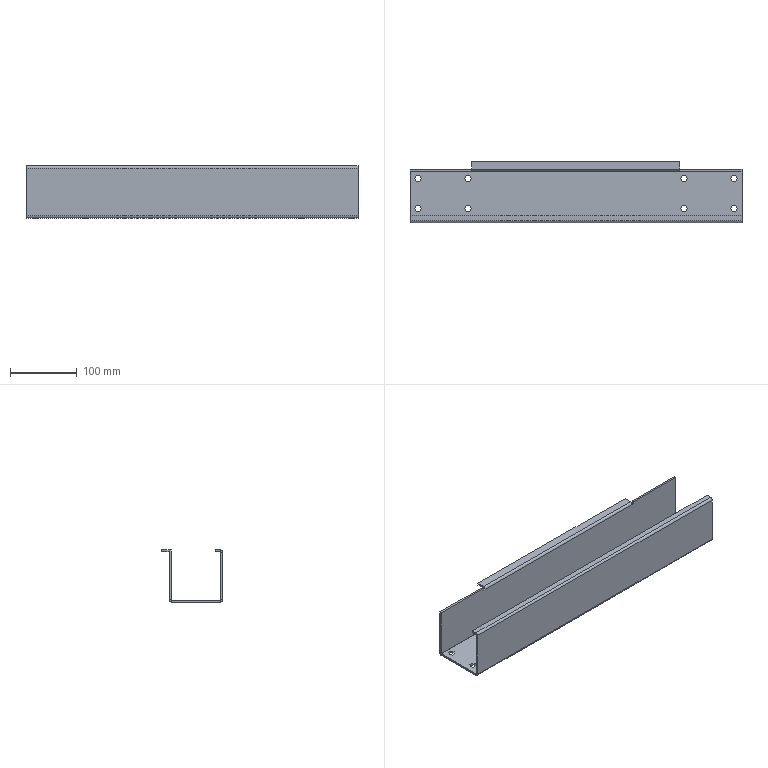Part | STEP file | 1 solid | 92 faces | box 498 x 92 x 78 mm | volume 361072 mm3 | plane 84 | cylinder 8 | commonest cylinder face diameters 0.4 x4 6.4 x4